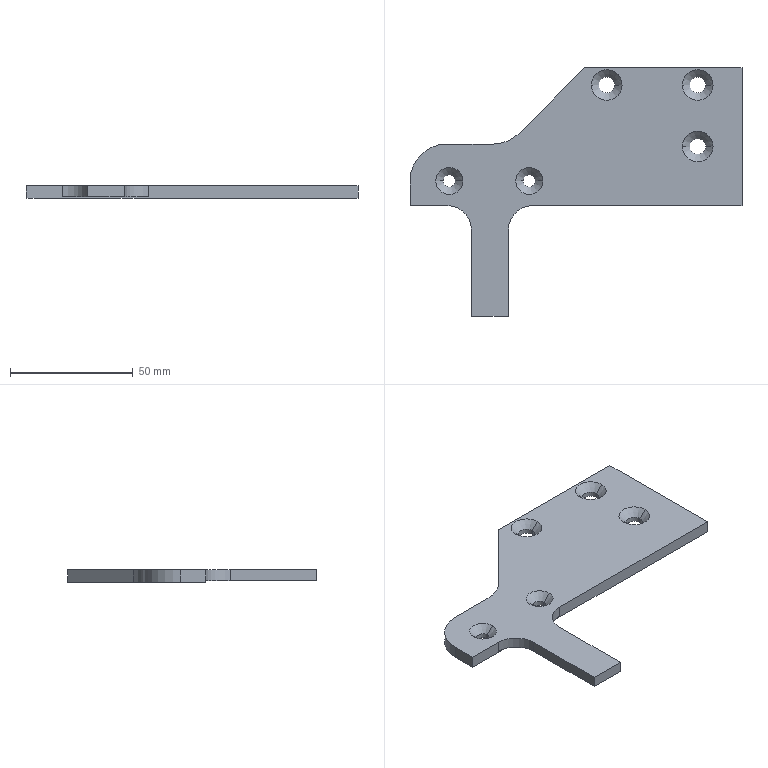Part | STEP file | Ngam kep 1M | 1 solid | 36 faces | box 135 x 101 x 5 mm | volume 30958 mm3 | cylinder 14 | plane 12 | cone 10 | commonest cylinder face diameters 6.5 x6 5 x4 20 x2 30 x2